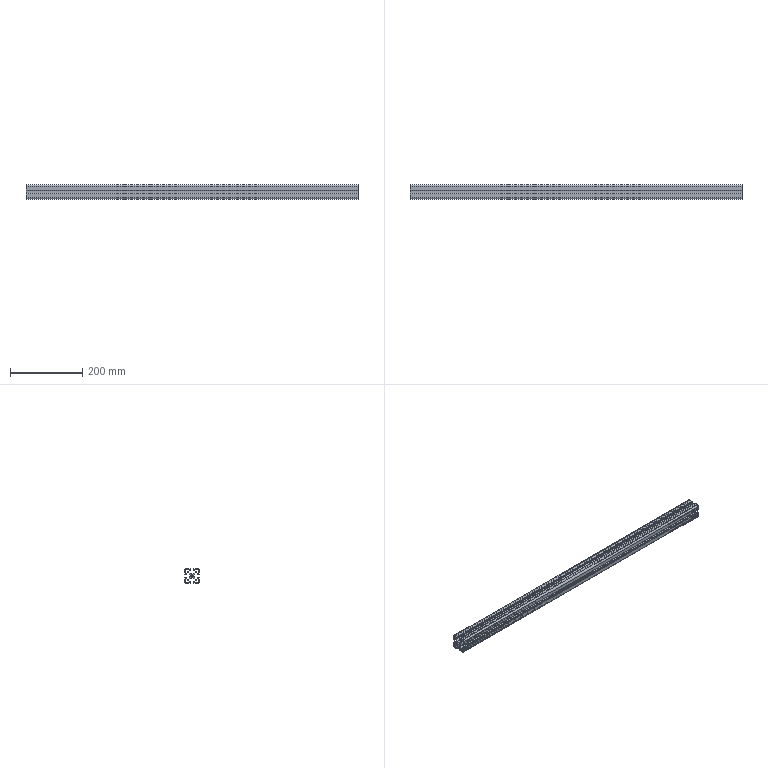Part | STEP file | MK-8-4040C-L-00 Profile 4040C Standard 920mm | 1 solid | 188 faces | box 920 x 40 x 40 mm | volume 439989 mm3 | cylinder 94 | plane 94 | commonest cylinder face diameters 0.6 x30 2 x28 4 x16 0.4 x8 6 x4 9 x4